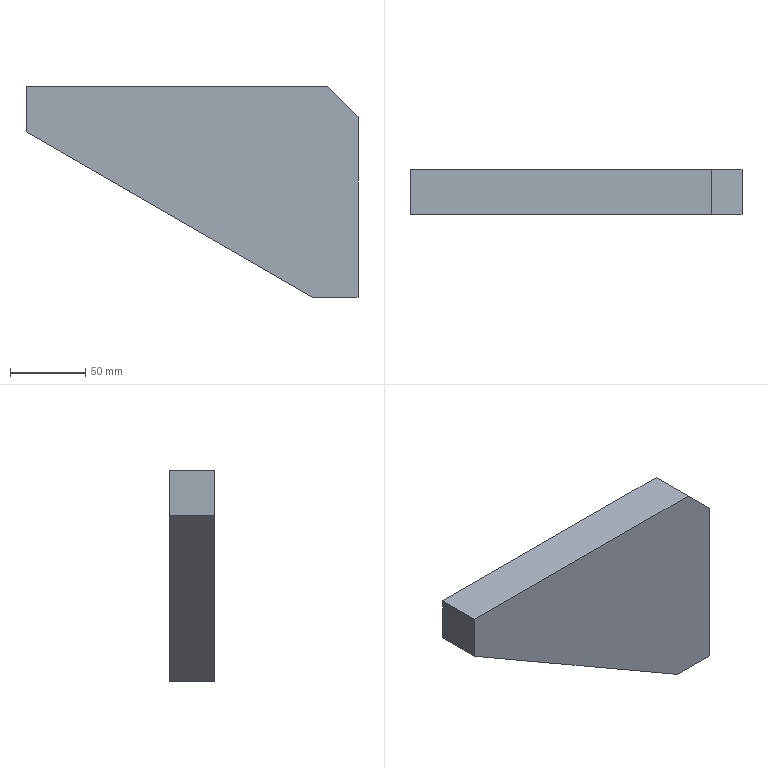Part | SolidWorks | features Extrusion 1 | 1 solid | 8 faces | box 220 x 30 x 139.697 mm | volume 603362 mm3 | plane 8
STEP:
#1=CARTESIAN_POINT('',(0.,0.,119.697));
#2=VERTEX_POINT('',#1);
#3=CARTESIAN_POINT('',(0.,0.,0.));
#4=VERTEX_POINT('',#3);
#5=CARTESIAN_POINT('',(0.,0.,119.697));
#6=DIRECTION('',(0.,0.,-1.));
#7=VECTOR('',#6,1000.);
#8=LINE('',#5,#7);
#9=EDGE_CURVE('',#2,#4,#8,.T.);
#10=ORIENTED_EDGE('',*,*,#9,.T.);
#11=CARTESIAN_POINT('',(0.,30.,0.));
#12=VERTEX_POINT('',#11);
#13=CARTESIAN_POINT('',(0.,30.,0.));
#14=DIRECTION('',(0.,-1.,0.));
#15=VECTOR('',#14,1000.);
#16=LINE('',#13,#15);
#17=EDGE_CURVE('',#12,#4,#16,.T.);
#18=ORIENTED_EDGE('',*,*,#17,.F.);
#19=CARTESIAN_POINT('',(0.,30.,119.697));
#20=VERTEX_POINT('',#19);
#21=CARTESIAN_POINT('',(0.,30.,119.697));
#22=DIRECTION('',(0.,0.,-1.));
#23=VECTOR('',#22,1000.);
#24=LINE('',#21,#23);
#25=EDGE_CURVE('',#20,#12,#24,.T.);
#26=ORIENTED_EDGE('',*,*,#25,.F.);
#27=CARTESIAN_POINT('',(0.,30.,119.697));
#28=DIRECTION('',(0.,-1.,0.));
#29=VECTOR('',#28,1000.);
#30=LINE('',#27,#29);
#31=EDGE_CURVE('',#20,#2,#30,.T.);
#32=ORIENTED_EDGE('',*,*,#31,.T.);
#33=EDGE_LOOP('',(#10,#18,#26,#32));
#34=FACE_OUTER_BOUND('',#33,.T.);
#35=CARTESIAN_POINT('',(0.,30.,119.697));
#36=DIRECTION('',(-1.,0.,0.));
#37=DIRECTION('',(0.,0.,1.));
#38=AXIS2_PLACEMENT_3D('',#35,#36,#37);
#39=PLANE('',#38);
#40=ADVANCED_FACE('',(#34),#39,.F.);
#41=CARTESIAN_POINT('',(-30.,0.,0.));
#42=VERTEX_POINT('',#41);
#43=CARTESIAN_POINT('',(0.,0.,0.));
#44=DIRECTION('',(-1.,0.,0.));
#45=VECTOR('',#44,1000.);
#46=LINE('',#43,#45);
#47=EDGE_CURVE('',#4,#42,#46,.T.);
#48=ORIENTED_EDGE('',*,*,#47,.T.);
#49=CARTESIAN_POINT('',(-30.,30.,0.));
#50=VERTEX_POINT('',#49);
#51=CARTESIAN_POINT('',(-30.,30.,0.));
#52=DIRECTION('',(0.,-1.,0.));
#53=VECTOR('',#52,1000.);
#54=LINE('',#51,#53);
#55=EDGE_CURVE('',#50,#42,#54,.T.);
#56=ORIENTED_EDGE('',*,*,#55,.F.);
#57=CARTESIAN_POINT('',(0.,30.,0.));
#58=DIRECTION('',(-1.,0.,0.));
#59=VECTOR('',#58,1000.);
#60=LINE('',#57,#59);
#61=EDGE_CURVE('',#12,#50,#60,.T.);
#62=ORIENTED_EDGE('',*,*,#61,.F.);
#63=ORIENTED_EDGE('',*,*,#17,.T.);
#64=EDGE_LOOP('',(#48,#56,#62,#63));
#65=FACE_OUTER_BOUND('',#64,.T.);
#66=CARTESIAN_POINT('',(0.,30.,0.));
#67=DIRECTION('',(0.,0.,1.));
#68=DIRECTION('',(1.,0.,0.));
#69=AXIS2_PLACEMENT_3D('',#66,#67,#68);
#70=PLANE('',#69);
#71=ADVANCED_FACE('',(#65),#70,.F.);
#72=CARTESIAN_POINT('',(-220.,0.,109.697));
#73=VERTEX_POINT('',#72);
#74=CARTESIAN_POINT('',(-30.,0.,0.));
#75=DIRECTION('',(-0.866,0.,0.5));
#76=VECTOR('',#75,1000.);
#77=LINE('',#74,#76);
#78=EDGE_CURVE('',#42,#73,#77,.T.);
#79=ORIENTED_EDGE('',*,*,#78,.T.);
#80=CARTESIAN_POINT('',(-220.,30.,109.697));
#81=VERTEX_POINT('',#80);
#82=CARTESIAN_POINT('',(-220.,30.,109.697));
#83=DIRECTION('',(0.,-1.,0.));
#84=VECTOR('',#83,1000.);
#85=LINE('',#82,#84);
#86=EDGE_CURVE('',#81,#73,#85,.T.);
#87=ORIENTED_EDGE('',*,*,#86,.F.);
#88=CARTESIAN_POINT('',(-30.,30.,0.));
#89=DIRECTION('',(-0.866,0.,0.5));
#90=VECTOR('',#89,1000.);
#91=LINE('',#88,#90);
#92=EDGE_CURVE('',#50,#81,#91,.T.);
#93=ORIENTED_EDGE('',*,*,#92,.F.);
#94=ORIENTED_EDGE('',*,*,#55,.T.);
#95=EDGE_LOOP('',(#79,#87,#93,#94));
#96=FACE_OUTER_BOUND('',#95,.T.);
#97=CARTESIAN_POINT('',(-30.,30.,0.));
#98=DIRECTION('',(0.5,0.,0.866));
#99=DIRECTION('',(0.866,0.,-0.5));
#100=AXIS2_PLACEMENT_3D('',#97,#98,#99);
#101=PLANE('',#100);
#102=ADVANCED_FACE('',(#96),#101,.F.);
#103=CARTESIAN_POINT('',(-220.,0.,139.697));
#104=VERTEX_POINT('',#103);
#105=CARTESIAN_POINT('',(-220.,0.,109.697));
#106=DIRECTION('',(0.,0.,1.));
#107=VECTOR('',#106,1000.);
#108=LINE('',#105,#107);
#109=EDGE_CURVE('',#73,#104,#108,.T.);
#110=ORIENTED_EDGE('',*,*,#109,.T.);
#111=CARTESIAN_POINT('',(-220.,30.,139.697));
#112=VERTEX_POINT('',#111);
#113=CARTESIAN_POINT('',(-220.,30.,139.697));
#114=DIRECTION('',(0.,-1.,0.));
#115=VECTOR('',#114,1000.);
#116=LINE('',#113,#115);
#117=EDGE_CURVE('',#112,#104,#116,.T.);
#118=ORIENTED_EDGE('',*,*,#117,.F.);
#119=CARTESIAN_POINT('',(-220.,30.,109.697));
#120=DIRECTION('',(0.,0.,1.));
#121=VECTOR('',#120,1000.);
#122=LINE('',#119,#121);
#123=EDGE_CURVE('',#81,#112,#122,.T.);
#124=ORIENTED_EDGE('',*,*,#123,.F.);
#125=ORIENTED_EDGE('',*,*,#86,.T.);
#126=EDGE_LOOP('',(#110,#118,#124,#125));
#127=FACE_OUTER_BOUND('',#126,.T.);
#128=CARTESIAN_POINT('',(-220.,30.,109.697));
#129=DIRECTION('',(1.,0.,0.));
#130=DIRECTION('',(0.,0.,-1.));
#131=AXIS2_PLACEMENT_3D('',#128,#129,#130);
#132=PLANE('',#131);
#133=ADVANCED_FACE('',(#127),#132,.F.);
#134=CARTESIAN_POINT('',(-20.,0.,139.697));
#135=VERTEX_POINT('',#134);
#136=CARTESIAN_POINT('',(-220.,0.,139.697));
#137=DIRECTION('',(1.,0.,0.));
#138=VECTOR('',#137,1000.);
#139=LINE('',#136,#138);
#140=EDGE_CURVE('',#104,#135,#139,.T.);
#141=ORIENTED_EDGE('',*,*,#140,.T.);
#142=CARTESIAN_POINT('',(-20.,30.,139.697));
#143=VERTEX_POINT('',#142);
#144=CARTESIAN_POINT('',(-20.,30.,139.697));
#145=DIRECTION('',(0.,-1.,0.));
#146=VECTOR('',#145,1000.);
#147=LINE('',#144,#146);
#148=EDGE_CURVE('',#143,#135,#147,.T.);
#149=ORIENTED_EDGE('',*,*,#148,.F.);
#150=CARTESIAN_POINT('',(-220.,30.,139.697));
#151=DIRECTION('',(1.,0.,0.));
#152=VECTOR('',#151,1000.);
#153=LINE('',#150,#152);
#154=EDGE_CURVE('',#112,#143,#153,.T.);
#155=ORIENTED_EDGE('',*,*,#154,.F.);
#156=ORIENTED_EDGE('',*,*,#117,.T.);
#157=EDGE_LOOP('',(#141,#149,#155,#156));
#158=FACE_OUTER_BOUND('',#157,.T.);
#159=CARTESIAN_POINT('',(-220.,30.,139.697));
#160=DIRECTION('',(0.,0.,-1.));
#161=DIRECTION('',(-1.,0.,0.));
#162=AXIS2_PLACEMENT_3D('',#159,#160,#161);
#163=PLANE('',#162);
#164=ADVANCED_FACE('',(#158),#163,.F.);
#165=CARTESIAN_POINT('',(-20.,0.,139.697));
#166=DIRECTION('',(0.7071,0.,-0.7071));
#167=VECTOR('',#166,1000.);
#168=LINE('',#165,#167);
#169=EDGE_CURVE('',#135,#2,#168,.T.);
#170=ORIENTED_EDGE('',*,*,#169,.T.);
#171=ORIENTED_EDGE('',*,*,#31,.F.);
#172=CARTESIAN_POINT('',(-20.,30.,139.697));
#173=DIRECTION('',(0.7071,0.,-0.7071));
#174=VECTOR('',#173,1000.);
#175=LINE('',#172,#174);
#176=EDGE_CURVE('',#143,#20,#175,.T.);
#177=ORIENTED_EDGE('',*,*,#176,.F.);
#178=ORIENTED_EDGE('',*,*,#148,.T.);
#179=EDGE_LOOP('',(#170,#171,#177,#178));
#180=FACE_OUTER_BOUND('',#179,.T.);
#181=CARTESIAN_POINT('',(-20.,30.,139.697));
#182=DIRECTION('',(-0.7071,0.,-0.7071));
#183=DIRECTION('',(-0.7071,0.,0.7071));
#184=AXIS2_PLACEMENT_3D('',#181,#182,#183);
#185=PLANE('',#184);
#186=ADVANCED_FACE('',(#180),#185,.F.);
#187=ORIENTED_EDGE('',*,*,#25,.T.);
#188=ORIENTED_EDGE('',*,*,#61,.T.);
#189=ORIENTED_EDGE('',*,*,#92,.T.);
#190=ORIENTED_EDGE('',*,*,#123,.T.);
#191=ORIENTED_EDGE('',*,*,#154,.T.);
#192=ORIENTED_EDGE('',*,*,#176,.T.);
#193=EDGE_LOOP('',(#187,#188,#189,#190,#191,#192));
#194=FACE_OUTER_BOUND('',#193,.T.);
#195=CARTESIAN_POINT('',(0.,30.,0.));
#196=DIRECTION('',(0.,1.,0.));
#197=DIRECTION('',(0.,0.,1.));
#198=AXIS2_PLACEMENT_3D('',#195,#196,#197);
#199=PLANE('',#198);
#200=ADVANCED_FACE('',(#194),#199,.T.);
#201=ORIENTED_EDGE('',*,*,#9,.F.);
#202=ORIENTED_EDGE('',*,*,#169,.F.);
#203=ORIENTED_EDGE('',*,*,#140,.F.);
#204=ORIENTED_EDGE('',*,*,#109,.F.);
#205=ORIENTED_EDGE('',*,*,#78,.F.);
#206=ORIENTED_EDGE('',*,*,#47,.F.);
#207=EDGE_LOOP('',(#201,#202,#203,#204,#205,#206));
#208=FACE_OUTER_BOUND('',#207,.T.);
#209=CARTESIAN_POINT('',(0.,0.,0.));
#210=DIRECTION('',(0.,1.,0.));
#211=DIRECTION('',(0.,0.,1.));
#212=AXIS2_PLACEMENT_3D('',#209,#210,#211);
#213=PLANE('',#212);
#214=ADVANCED_FACE('',(#208),#213,.F.);
#215=CLOSED_SHELL('',(#40,#71,#102,#133,#164,#186,#200,#214));
#216=MANIFOLD_SOLID_BREP('',#215);
#217=CARTESIAN_POINT('',(0.,0.,0.));
#218=DIRECTION('',(0.,0.,1.));
#219=DIRECTION('',(1.,0.,0.));
#220=AXIS2_PLACEMENT_3D('',#217,#218,#219);
#221=(LENGTH_UNIT()NAMED_UNIT(*)SI_UNIT(.MILLI.,.METRE.));
#222=UNCERTAINTY_MEASURE_WITH_UNIT(LENGTH_MEASURE(0.00001),#221,'','');
#223=(NAMED_UNIT(*)PLANE_ANGLE_UNIT()SI_UNIT($,.RADIAN.));
#224=(NAMED_UNIT(*)SI_UNIT($,.STERADIAN.)SOLID_ANGLE_UNIT());
#225=(GEOMETRIC_REPRESENTATION_CONTEXT(3)GLOBAL_UNCERTAINTY_ASSIGNED_CONTEXT((#222))GLOBAL_UNIT_ASSIGNED_CONTEXT((#221,#223,#224))REPRESENTATION_CONTEXT('',''));
#226=ADVANCED_BREP_SHAPE_REPRESENTATION('',(#216,#220),#225);